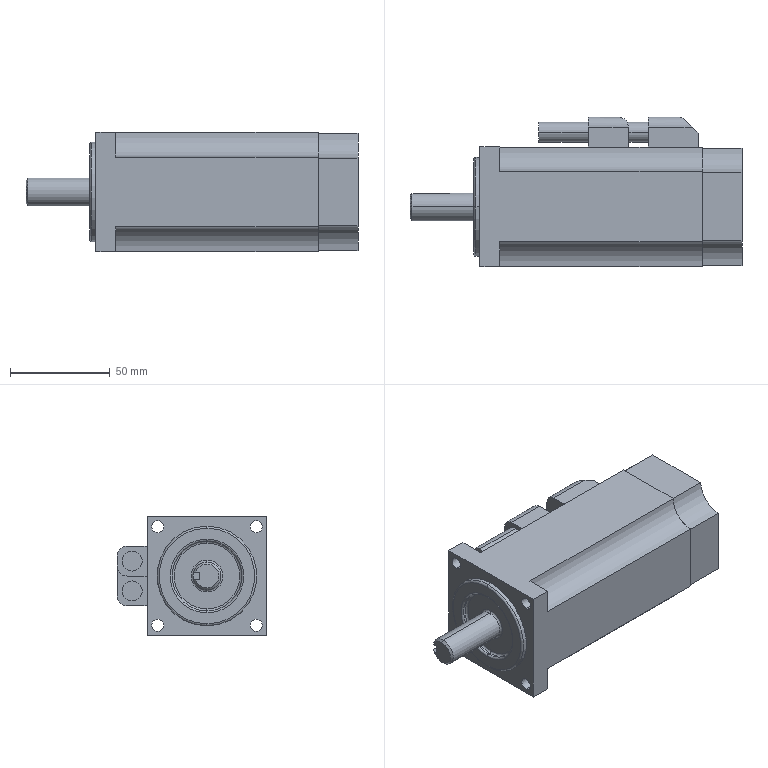Part | NX | 1 solid | 78 faces | box 166.5 x 75 x 60 mm | volume 436782 mm3 | plane 35 | cylinder 32 | torus 8 | cone 3 | commonest cylinder face diameters 10 x10 6 x8 25 x4 26 x4 14 x2 35 x2